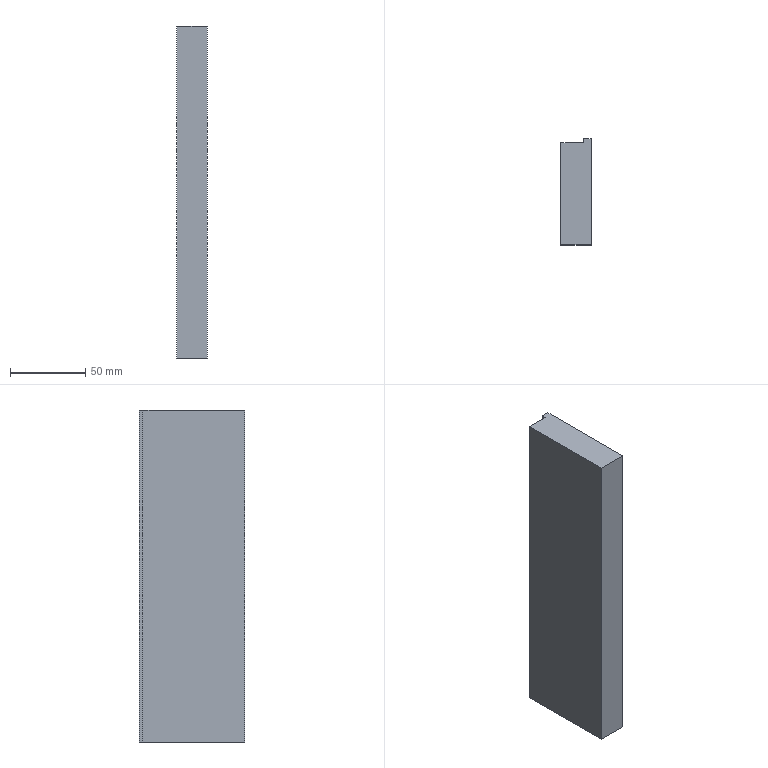Part | STEP file | Backup 2012-3-22-015 | 1 solid | 8 faces | box 20 x 70 x 220 mm | volume 299750 mm3 | plane 8
STEP:
#1=CARTESIAN_POINT('',(0.,0.,0.));
#2=DIRECTION('',(0.,0.,1.));
#3=DIRECTION('',(1.,0.,0.));
#4=AXIS2_PLACEMENT_3D('',#1,#2,#3);
#5=CARTESIAN_POINT('',(0.,67.5,0.));
#6=VERTEX_POINT('',#5);
#7=CARTESIAN_POINT('',(0.,0.,0.));
#8=VERTEX_POINT('',#7);
#9=CARTESIAN_POINT('',(0.,0.,0.));
#10=DIRECTION('',(0.,-1.,0.));
#11=VECTOR('',#10,1.);
#12=LINE('',#9,#11);
#13=CARTESIAN_POINT('',(0.,0.,220.));
#14=DIRECTION('',(1.,0.,0.));
#15=DIRECTION('',(0.,0.,-1.));
#16=AXIS2_PLACEMENT_3D('',#13,#14,#15);
#17=PLANE('',#16);
#18=CARTESIAN_POINT('',(220.,0.));
#19=DIRECTION('',(0.,-1.));
#20=VECTOR('',#19,1.);
#21=LINE('',#18,#20);
#22=(GEOMETRIC_REPRESENTATION_CONTEXT(2)PARAMETRIC_REPRESENTATION_CONTEXT()REPRESENTATION_CONTEXT('',''));
#23=DEFINITIONAL_REPRESENTATION('',(#21),#22);
#24=PCURVE('',#17,#23);
#25=CARTESIAN_POINT('',(0.,67.5,0.));
#26=DIRECTION('',(0.,0.,1.));
#27=DIRECTION('',(1.,0.,0.));
#28=AXIS2_PLACEMENT_3D('',#25,#26,#27);
#29=PLANE('',#28);
#30=CARTESIAN_POINT('',(0.,-67.5));
#31=DIRECTION('',(0.,-1.));
#32=VECTOR('',#31,1.);
#33=LINE('',#30,#32);
#34=(GEOMETRIC_REPRESENTATION_CONTEXT(2)PARAMETRIC_REPRESENTATION_CONTEXT()REPRESENTATION_CONTEXT('',''));
#35=DEFINITIONAL_REPRESENTATION('',(#33),#34);
#36=PCURVE('',#29,#35);
#37=SURFACE_CURVE('',#12,(#24,#36),.PCURVE_S1.);
#38=EDGE_CURVE('',#6,#8,#37,.T.);
#39=ORIENTED_EDGE('',*,*,#38,.T.);
#40=CARTESIAN_POINT('',(0.,0.,220.));
#41=VERTEX_POINT('',#40);
#42=CARTESIAN_POINT('',(0.,0.,220.));
#43=DIRECTION('',(0.,0.,-1.));
#44=VECTOR('',#43,1.);
#45=LINE('',#42,#44);
#46=CARTESIAN_POINT('',(0.,0.));
#47=DIRECTION('',(1.,0.));
#48=VECTOR('',#47,1.);
#49=LINE('',#46,#48);
#50=(GEOMETRIC_REPRESENTATION_CONTEXT(2)PARAMETRIC_REPRESENTATION_CONTEXT()REPRESENTATION_CONTEXT('',''));
#51=DEFINITIONAL_REPRESENTATION('',(#49),#50);
#52=PCURVE('',#17,#51);
#53=CARTESIAN_POINT('',(0.,0.,220.));
#54=DIRECTION('',(0.,1.,0.));
#55=DIRECTION('',(0.,0.,1.));
#56=AXIS2_PLACEMENT_3D('',#53,#54,#55);
#57=PLANE('',#56);
#58=CARTESIAN_POINT('',(0.,0.));
#59=DIRECTION('',(-1.,0.));
#60=VECTOR('',#59,1.);
#61=LINE('',#58,#60);
#62=(GEOMETRIC_REPRESENTATION_CONTEXT(2)PARAMETRIC_REPRESENTATION_CONTEXT()REPRESENTATION_CONTEXT('',''));
#63=DEFINITIONAL_REPRESENTATION('',(#61),#62);
#64=PCURVE('',#57,#63);
#65=SURFACE_CURVE('',#45,(#52,#64),.PCURVE_S1.);
#66=EDGE_CURVE('',#41,#8,#65,.T.);
#67=ORIENTED_EDGE('',*,*,#66,.F.);
#68=CARTESIAN_POINT('',(0.,67.5,220.));
#69=VERTEX_POINT('',#68);
#70=CARTESIAN_POINT('',(0.,0.,220.));
#71=DIRECTION('',(0.,-1.,0.));
#72=VECTOR('',#71,1.);
#73=LINE('',#70,#72);
#74=CARTESIAN_POINT('',(0.,0.));
#75=DIRECTION('',(0.,-1.));
#76=VECTOR('',#75,1.);
#77=LINE('',#74,#76);
#78=(GEOMETRIC_REPRESENTATION_CONTEXT(2)PARAMETRIC_REPRESENTATION_CONTEXT()REPRESENTATION_CONTEXT('',''));
#79=DEFINITIONAL_REPRESENTATION('',(#77),#78);
#80=PCURVE('',#17,#79);
#81=CARTESIAN_POINT('',(0.,67.5,220.));
#82=DIRECTION('',(0.,0.,1.));
#83=DIRECTION('',(1.,0.,0.));
#84=AXIS2_PLACEMENT_3D('',#81,#82,#83);
#85=PLANE('',#84);
#86=CARTESIAN_POINT('',(0.,-67.5));
#87=DIRECTION('',(0.,-1.));
#88=VECTOR('',#87,1.);
#89=LINE('',#86,#88);
#90=(GEOMETRIC_REPRESENTATION_CONTEXT(2)PARAMETRIC_REPRESENTATION_CONTEXT()REPRESENTATION_CONTEXT('',''));
#91=DEFINITIONAL_REPRESENTATION('',(#89),#90);
#92=PCURVE('',#85,#91);
#93=SURFACE_CURVE('',#73,(#80,#92),.PCURVE_S1.);
#94=EDGE_CURVE('',#69,#41,#93,.T.);
#95=ORIENTED_EDGE('',*,*,#94,.F.);
#96=CARTESIAN_POINT('',(0.,67.5,220.));
#97=DIRECTION('',(0.,0.,-1.));
#98=VECTOR('',#97,1.);
#99=LINE('',#96,#98);
#100=CARTESIAN_POINT('',(0.,67.5));
#101=DIRECTION('',(1.,0.));
#102=VECTOR('',#101,1.);
#103=LINE('',#100,#102);
#104=(GEOMETRIC_REPRESENTATION_CONTEXT(2)PARAMETRIC_REPRESENTATION_CONTEXT()REPRESENTATION_CONTEXT('',''));
#105=DEFINITIONAL_REPRESENTATION('',(#103),#104);
#106=PCURVE('',#17,#105);
#107=CARTESIAN_POINT('',(15.,67.5,220.));
#108=DIRECTION('',(0.,-1.,0.));
#109=DIRECTION('',(0.,0.,-1.));
#110=AXIS2_PLACEMENT_3D('',#107,#108,#109);
#111=PLANE('',#110);
#112=CARTESIAN_POINT('',(0.,-15.));
#113=DIRECTION('',(1.,0.));
#114=VECTOR('',#113,1.);
#115=LINE('',#112,#114);
#116=(GEOMETRIC_REPRESENTATION_CONTEXT(2)PARAMETRIC_REPRESENTATION_CONTEXT()REPRESENTATION_CONTEXT('',''));
#117=DEFINITIONAL_REPRESENTATION('',(#115),#116);
#118=PCURVE('',#111,#117);
#119=SURFACE_CURVE('',#99,(#106,#118),.PCURVE_S1.);
#120=EDGE_CURVE('',#69,#6,#119,.T.);
#121=ORIENTED_EDGE('',*,*,#120,.T.);
#122=EDGE_LOOP('',(#39,#67,#95,#121));
#123=FACE_BOUND('',#122,.T.);
#124=ADVANCED_FACE('',(#123),#17,.F.);
#125=CARTESIAN_POINT('',(20.,0.,0.));
#126=VERTEX_POINT('',#125);
#127=CARTESIAN_POINT('',(0.,0.,0.));
#128=DIRECTION('',(1.,0.,0.));
#129=VECTOR('',#128,1.);
#130=LINE('',#127,#129);
#131=CARTESIAN_POINT('',(-220.,0.));
#132=DIRECTION('',(0.,1.));
#133=VECTOR('',#132,1.);
#134=LINE('',#131,#133);
#135=(GEOMETRIC_REPRESENTATION_CONTEXT(2)PARAMETRIC_REPRESENTATION_CONTEXT()REPRESENTATION_CONTEXT('',''));
#136=DEFINITIONAL_REPRESENTATION('',(#134),#135);
#137=PCURVE('',#57,#136);
#138=CARTESIAN_POINT('',(0.,-67.5));
#139=DIRECTION('',(1.,0.));
#140=VECTOR('',#139,1.);
#141=LINE('',#138,#140);
#142=(GEOMETRIC_REPRESENTATION_CONTEXT(2)PARAMETRIC_REPRESENTATION_CONTEXT()REPRESENTATION_CONTEXT('',''));
#143=DEFINITIONAL_REPRESENTATION('',(#141),#142);
#144=PCURVE('',#29,#143);
#145=SURFACE_CURVE('',#130,(#137,#144),.PCURVE_S1.);
#146=EDGE_CURVE('',#8,#126,#145,.T.);
#147=ORIENTED_EDGE('',*,*,#146,.T.);
#148=CARTESIAN_POINT('',(20.,0.,220.));
#149=VERTEX_POINT('',#148);
#150=CARTESIAN_POINT('',(20.,0.,220.));
#151=DIRECTION('',(0.,0.,-1.));
#152=VECTOR('',#151,1.);
#153=LINE('',#150,#152);
#154=CARTESIAN_POINT('',(0.,20.));
#155=DIRECTION('',(-1.,0.));
#156=VECTOR('',#155,1.);
#157=LINE('',#154,#156);
#158=(GEOMETRIC_REPRESENTATION_CONTEXT(2)PARAMETRIC_REPRESENTATION_CONTEXT()REPRESENTATION_CONTEXT('',''));
#159=DEFINITIONAL_REPRESENTATION('',(#157),#158);
#160=PCURVE('',#57,#159);
#161=CARTESIAN_POINT('',(20.,0.,220.));
#162=DIRECTION('',(-1.,0.,0.));
#163=DIRECTION('',(0.,-1.,0.));
#164=AXIS2_PLACEMENT_3D('',#161,#162,#163);
#165=PLANE('',#164);
#166=CARTESIAN_POINT('',(0.,0.));
#167=DIRECTION('',(0.,-1.));
#168=VECTOR('',#167,1.);
#169=LINE('',#166,#168);
#170=(GEOMETRIC_REPRESENTATION_CONTEXT(2)PARAMETRIC_REPRESENTATION_CONTEXT()REPRESENTATION_CONTEXT('',''));
#171=DEFINITIONAL_REPRESENTATION('',(#169),#170);
#172=PCURVE('',#165,#171);
#173=SURFACE_CURVE('',#153,(#160,#172),.PCURVE_S1.);
#174=EDGE_CURVE('',#149,#126,#173,.T.);
#175=ORIENTED_EDGE('',*,*,#174,.F.);
#176=CARTESIAN_POINT('',(0.,0.,220.));
#177=DIRECTION('',(1.,0.,0.));
#178=VECTOR('',#177,1.);
#179=LINE('',#176,#178);
#180=CARTESIAN_POINT('',(0.,0.));
#181=DIRECTION('',(0.,1.));
#182=VECTOR('',#181,1.);
#183=LINE('',#180,#182);
#184=(GEOMETRIC_REPRESENTATION_CONTEXT(2)PARAMETRIC_REPRESENTATION_CONTEXT()REPRESENTATION_CONTEXT('',''));
#185=DEFINITIONAL_REPRESENTATION('',(#183),#184);
#186=PCURVE('',#57,#185);
#187=CARTESIAN_POINT('',(0.,-67.5));
#188=DIRECTION('',(1.,0.));
#189=VECTOR('',#188,1.);
#190=LINE('',#187,#189);
#191=(GEOMETRIC_REPRESENTATION_CONTEXT(2)PARAMETRIC_REPRESENTATION_CONTEXT()REPRESENTATION_CONTEXT('',''));
#192=DEFINITIONAL_REPRESENTATION('',(#190),#191);
#193=PCURVE('',#85,#192);
#194=SURFACE_CURVE('',#179,(#186,#193),.PCURVE_S1.);
#195=EDGE_CURVE('',#41,#149,#194,.T.);
#196=ORIENTED_EDGE('',*,*,#195,.F.);
#197=ORIENTED_EDGE('',*,*,#66,.T.);
#198=EDGE_LOOP('',(#147,#175,#196,#197));
#199=FACE_BOUND('',#198,.T.);
#200=ADVANCED_FACE('',(#199),#57,.F.);
#201=CARTESIAN_POINT('',(20.,70.,0.));
#202=VERTEX_POINT('',#201);
#203=CARTESIAN_POINT('',(20.,0.,0.));
#204=DIRECTION('',(0.,1.,0.));
#205=VECTOR('',#204,1.);
#206=LINE('',#203,#205);
#207=CARTESIAN_POINT('',(0.,-220.));
#208=DIRECTION('',(-1.,0.));
#209=VECTOR('',#208,1.);
#210=LINE('',#207,#209);
#211=(GEOMETRIC_REPRESENTATION_CONTEXT(2)PARAMETRIC_REPRESENTATION_CONTEXT()REPRESENTATION_CONTEXT('',''));
#212=DEFINITIONAL_REPRESENTATION('',(#210),#211);
#213=PCURVE('',#165,#212);
#214=CARTESIAN_POINT('',(20.,-67.5));
#215=DIRECTION('',(0.,1.));
#216=VECTOR('',#215,1.);
#217=LINE('',#214,#216);
#218=(GEOMETRIC_REPRESENTATION_CONTEXT(2)PARAMETRIC_REPRESENTATION_CONTEXT()REPRESENTATION_CONTEXT('',''));
#219=DEFINITIONAL_REPRESENTATION('',(#217),#218);
#220=PCURVE('',#29,#219);
#221=SURFACE_CURVE('',#206,(#213,#220),.PCURVE_S1.);
#222=EDGE_CURVE('',#126,#202,#221,.T.);
#223=ORIENTED_EDGE('',*,*,#222,.T.);
#224=CARTESIAN_POINT('',(20.,70.,220.));
#225=VERTEX_POINT('',#224);
#226=CARTESIAN_POINT('',(20.,70.,220.));
#227=DIRECTION('',(0.,0.,-1.));
#228=VECTOR('',#227,1.);
#229=LINE('',#226,#228);
#230=CARTESIAN_POINT('',(-70.,0.));
#231=DIRECTION('',(0.,-1.));
#232=VECTOR('',#231,1.);
#233=LINE('',#230,#232);
#234=(GEOMETRIC_REPRESENTATION_CONTEXT(2)PARAMETRIC_REPRESENTATION_CONTEXT()REPRESENTATION_CONTEXT('',''));
#235=DEFINITIONAL_REPRESENTATION('',(#233),#234);
#236=PCURVE('',#165,#235);
#237=CARTESIAN_POINT('',(15.,70.,220.));
#238=DIRECTION('',(0.,-1.,0.));
#239=DIRECTION('',(0.,0.,-1.));
#240=AXIS2_PLACEMENT_3D('',#237,#238,#239);
#241=PLANE('',#240);
#242=CARTESIAN_POINT('',(0.,5.));
#243=DIRECTION('',(1.,0.));
#244=VECTOR('',#243,1.);
#245=LINE('',#242,#244);
#246=(GEOMETRIC_REPRESENTATION_CONTEXT(2)PARAMETRIC_REPRESENTATION_CONTEXT()REPRESENTATION_CONTEXT('',''));
#247=DEFINITIONAL_REPRESENTATION('',(#245),#246);
#248=PCURVE('',#241,#247);
#249=SURFACE_CURVE('',#229,(#236,#248),.PCURVE_S1.);
#250=EDGE_CURVE('',#225,#202,#249,.T.);
#251=ORIENTED_EDGE('',*,*,#250,.F.);
#252=CARTESIAN_POINT('',(20.,0.,220.));
#253=DIRECTION('',(0.,1.,0.));
#254=VECTOR('',#253,1.);
#255=LINE('',#252,#254);
#256=CARTESIAN_POINT('',(0.,0.));
#257=DIRECTION('',(-1.,0.));
#258=VECTOR('',#257,1.);
#259=LINE('',#256,#258);
#260=(GEOMETRIC_REPRESENTATION_CONTEXT(2)PARAMETRIC_REPRESENTATION_CONTEXT()REPRESENTATION_CONTEXT('',''));
#261=DEFINITIONAL_REPRESENTATION('',(#259),#260);
#262=PCURVE('',#165,#261);
#263=CARTESIAN_POINT('',(20.,-67.5));
#264=DIRECTION('',(0.,1.));
#265=VECTOR('',#264,1.);
#266=LINE('',#263,#265);
#267=(GEOMETRIC_REPRESENTATION_CONTEXT(2)PARAMETRIC_REPRESENTATION_CONTEXT()REPRESENTATION_CONTEXT('',''));
#268=DEFINITIONAL_REPRESENTATION('',(#266),#267);
#269=PCURVE('',#85,#268);
#270=SURFACE_CURVE('',#255,(#262,#269),.PCURVE_S1.);
#271=EDGE_CURVE('',#149,#225,#270,.T.);
#272=ORIENTED_EDGE('',*,*,#271,.F.);
#273=ORIENTED_EDGE('',*,*,#174,.T.);
#274=EDGE_LOOP('',(#223,#251,#272,#273));
#275=FACE_BOUND('',#274,.T.);
#276=ADVANCED_FACE('',(#275),#165,.F.);
#277=CARTESIAN_POINT('',(15.,70.,0.));
#278=VERTEX_POINT('',#277);
#279=CARTESIAN_POINT('',(15.,70.,0.));
#280=DIRECTION('',(-1.,0.,0.));
#281=VECTOR('',#280,1.);
#282=LINE('',#279,#281);
#283=CARTESIAN_POINT('',(220.,0.));
#284=DIRECTION('',(0.,-1.));
#285=VECTOR('',#284,1.);
#286=LINE('',#283,#285);
#287=(GEOMETRIC_REPRESENTATION_CONTEXT(2)PARAMETRIC_REPRESENTATION_CONTEXT()REPRESENTATION_CONTEXT('',''));
#288=DEFINITIONAL_REPRESENTATION('',(#286),#287);
#289=PCURVE('',#241,#288);
#290=CARTESIAN_POINT('',(15.,2.5));
#291=DIRECTION('',(-1.,0.));
#292=VECTOR('',#291,1.);
#293=LINE('',#290,#292);
#294=(GEOMETRIC_REPRESENTATION_CONTEXT(2)PARAMETRIC_REPRESENTATION_CONTEXT()REPRESENTATION_CONTEXT('',''));
#295=DEFINITIONAL_REPRESENTATION('',(#293),#294);
#296=PCURVE('',#29,#295);
#297=SURFACE_CURVE('',#282,(#289,#296),.PCURVE_S1.);
#298=EDGE_CURVE('',#202,#278,#297,.T.);
#299=ORIENTED_EDGE('',*,*,#298,.T.);
#300=CARTESIAN_POINT('',(15.,70.,220.));
#301=VERTEX_POINT('',#300);
#302=CARTESIAN_POINT('',(15.,70.,220.));
#303=DIRECTION('',(0.,0.,-1.));
#304=VECTOR('',#303,1.);
#305=LINE('',#302,#304);
#306=CARTESIAN_POINT('',(0.,0.));
#307=DIRECTION('',(1.,0.));
#308=VECTOR('',#307,1.);
#309=LINE('',#306,#308);
#310=(GEOMETRIC_REPRESENTATION_CONTEXT(2)PARAMETRIC_REPRESENTATION_CONTEXT()REPRESENTATION_CONTEXT('',''));
#311=DEFINITIONAL_REPRESENTATION('',(#309),#310);
#312=PCURVE('',#241,#311);
#313=CARTESIAN_POINT('',(15.,70.,220.));
#314=DIRECTION('',(1.,0.,0.));
#315=DIRECTION('',(0.,0.,-1.));
#316=AXIS2_PLACEMENT_3D('',#313,#314,#315);
#317=PLANE('',#316);
#318=CARTESIAN_POINT('',(0.,0.));
#319=DIRECTION('',(1.,0.));
#320=VECTOR('',#319,1.);
#321=LINE('',#318,#320);
#322=(GEOMETRIC_REPRESENTATION_CONTEXT(2)PARAMETRIC_REPRESENTATION_CONTEXT()REPRESENTATION_CONTEXT('',''));
#323=DEFINITIONAL_REPRESENTATION('',(#321),#322);
#324=PCURVE('',#317,#323);
#325=SURFACE_CURVE('',#305,(#312,#324),.PCURVE_S1.);
#326=EDGE_CURVE('',#301,#278,#325,.T.);
#327=ORIENTED_EDGE('',*,*,#326,.F.);
#328=CARTESIAN_POINT('',(15.,70.,220.));
#329=DIRECTION('',(-1.,0.,0.));
#330=VECTOR('',#329,1.);
#331=LINE('',#328,#330);
#332=CARTESIAN_POINT('',(0.,0.));
#333=DIRECTION('',(0.,-1.));
#334=VECTOR('',#333,1.);
#335=LINE('',#332,#334);
#336=(GEOMETRIC_REPRESENTATION_CONTEXT(2)PARAMETRIC_REPRESENTATION_CONTEXT()REPRESENTATION_CONTEXT('',''));
#337=DEFINITIONAL_REPRESENTATION('',(#335),#336);
#338=PCURVE('',#241,#337);
#339=CARTESIAN_POINT('',(15.,2.5));
#340=DIRECTION('',(-1.,0.));
#341=VECTOR('',#340,1.);
#342=LINE('',#339,#341);
#343=(GEOMETRIC_REPRESENTATION_CONTEXT(2)PARAMETRIC_REPRESENTATION_CONTEXT()REPRESENTATION_CONTEXT('',''));
#344=DEFINITIONAL_REPRESENTATION('',(#342),#343);
#345=PCURVE('',#85,#344);
#346=SURFACE_CURVE('',#331,(#338,#345),.PCURVE_S1.);
#347=EDGE_CURVE('',#225,#301,#346,.T.);
#348=ORIENTED_EDGE('',*,*,#347,.F.);
#349=ORIENTED_EDGE('',*,*,#250,.T.);
#350=EDGE_LOOP('',(#299,#327,#348,#349));
#351=FACE_BOUND('',#350,.T.);
#352=ADVANCED_FACE('',(#351),#241,.F.);
#353=CARTESIAN_POINT('',(15.,67.5,0.));
#354=VERTEX_POINT('',#353);
#355=CARTESIAN_POINT('',(15.,70.,0.));
#356=DIRECTION('',(0.,-1.,0.));
#357=VECTOR('',#356,1.);
#358=LINE('',#355,#357);
#359=CARTESIAN_POINT('',(220.,0.));
#360=DIRECTION('',(0.,-1.));
#361=VECTOR('',#360,1.);
#362=LINE('',#359,#361);
#363=(GEOMETRIC_REPRESENTATION_CONTEXT(2)PARAMETRIC_REPRESENTATION_CONTEXT()REPRESENTATION_CONTEXT('',''));
#364=DEFINITIONAL_REPRESENTATION('',(#362),#363);
#365=PCURVE('',#317,#364);
#366=CARTESIAN_POINT('',(15.,2.5));
#367=DIRECTION('',(0.,-1.));
#368=VECTOR('',#367,1.);
#369=LINE('',#366,#368);
#370=(GEOMETRIC_REPRESENTATION_CONTEXT(2)PARAMETRIC_REPRESENTATION_CONTEXT()REPRESENTATION_CONTEXT('',''));
#371=DEFINITIONAL_REPRESENTATION('',(#369),#370);
#372=PCURVE('',#29,#371);
#373=SURFACE_CURVE('',#358,(#365,#372),.PCURVE_S1.);
#374=EDGE_CURVE('',#278,#354,#373,.T.);
#375=ORIENTED_EDGE('',*,*,#374,.T.);
#376=CARTESIAN_POINT('',(15.,67.5,220.));
#377=VERTEX_POINT('',#376);
#378=CARTESIAN_POINT('',(15.,67.5,220.));
#379=DIRECTION('',(0.,0.,-1.));
#380=VECTOR('',#379,1.);
#381=LINE('',#378,#380);
#382=CARTESIAN_POINT('',(0.,-2.5));
#383=DIRECTION('',(1.,0.));
#384=VECTOR('',#383,1.);
#385=LINE('',#382,#384);
#386=(GEOMETRIC_REPRESENTATION_CONTEXT(2)PARAMETRIC_REPRESENTATION_CONTEXT()REPRESENTATION_CONTEXT('',''));
#387=DEFINITIONAL_REPRESENTATION('',(#385),#386);
#388=PCURVE('',#317,#387);
#389=CARTESIAN_POINT('',(0.,0.));
#390=DIRECTION('',(1.,0.));
#391=VECTOR('',#390,1.);
#392=LINE('',#389,#391);
#393=(GEOMETRIC_REPRESENTATION_CONTEXT(2)PARAMETRIC_REPRESENTATION_CONTEXT()REPRESENTATION_CONTEXT('',''));
#394=DEFINITIONAL_REPRESENTATION('',(#392),#393);
#395=PCURVE('',#111,#394);
#396=SURFACE_CURVE('',#381,(#388,#395),.PCURVE_S1.);
#397=EDGE_CURVE('',#377,#354,#396,.T.);
#398=ORIENTED_EDGE('',*,*,#397,.F.);
#399=CARTESIAN_POINT('',(15.,70.,220.));
#400=DIRECTION('',(0.,-1.,0.));
#401=VECTOR('',#400,1.);
#402=LINE('',#399,#401);
#403=CARTESIAN_POINT('',(0.,0.));
#404=DIRECTION('',(0.,-1.));
#405=VECTOR('',#404,1.);
#406=LINE('',#403,#405);
#407=(GEOMETRIC_REPRESENTATION_CONTEXT(2)PARAMETRIC_REPRESENTATION_CONTEXT()REPRESENTATION_CONTEXT('',''));
#408=DEFINITIONAL_REPRESENTATION('',(#406),#407);
#409=PCURVE('',#317,#408);
#410=CARTESIAN_POINT('',(15.,2.5));
#411=DIRECTION('',(0.,-1.));
#412=VECTOR('',#411,1.);
#413=LINE('',#410,#412);
#414=(GEOMETRIC_REPRESENTATION_CONTEXT(2)PARAMETRIC_REPRESENTATION_CONTEXT()REPRESENTATION_CONTEXT('',''));
#415=DEFINITIONAL_REPRESENTATION('',(#413),#414);
#416=PCURVE('',#85,#415);
#417=SURFACE_CURVE('',#402,(#409,#416),.PCURVE_S1.);
#418=EDGE_CURVE('',#301,#377,#417,.T.);
#419=ORIENTED_EDGE('',*,*,#418,.F.);
#420=ORIENTED_EDGE('',*,*,#326,.T.);
#421=EDGE_LOOP('',(#375,#398,#419,#420));
#422=FACE_BOUND('',#421,.T.);
#423=ADVANCED_FACE('',(#422),#317,.F.);
#424=CARTESIAN_POINT('',(15.,67.5,0.));
#425=DIRECTION('',(-1.,0.,0.));
#426=VECTOR('',#425,1.);
#427=LINE('',#424,#426);
#428=CARTESIAN_POINT('',(220.,0.));
#429=DIRECTION('',(0.,-1.));
#430=VECTOR('',#429,1.);
#431=LINE('',#428,#430);
#432=(GEOMETRIC_REPRESENTATION_CONTEXT(2)PARAMETRIC_REPRESENTATION_CONTEXT()REPRESENTATION_CONTEXT('',''));
#433=DEFINITIONAL_REPRESENTATION('',(#431),#432);
#434=PCURVE('',#111,#433);
#435=CARTESIAN_POINT('',(15.,0.));
#436=DIRECTION('',(-1.,0.));
#437=VECTOR('',#436,1.);
#438=LINE('',#435,#437);
#439=(GEOMETRIC_REPRESENTATION_CONTEXT(2)PARAMETRIC_REPRESENTATION_CONTEXT()REPRESENTATION_CONTEXT('',''));
#440=DEFINITIONAL_REPRESENTATION('',(#438),#439);
#441=PCURVE('',#29,#440);
#442=SURFACE_CURVE('',#427,(#434,#441),.PCURVE_S1.);
#443=EDGE_CURVE('',#354,#6,#442,.T.);
#444=ORIENTED_EDGE('',*,*,#443,.T.);
#445=ORIENTED_EDGE('',*,*,#120,.F.);
#446=CARTESIAN_POINT('',(15.,67.5,220.));
#447=DIRECTION('',(-1.,0.,0.));
#448=VECTOR('',#447,1.);
#449=LINE('',#446,#448);
#450=CARTESIAN_POINT('',(0.,0.));
#451=DIRECTION('',(0.,-1.));
#452=VECTOR('',#451,1.);
#453=LINE('',#450,#452);
#454=(GEOMETRIC_REPRESENTATION_CONTEXT(2)PARAMETRIC_REPRESENTATION_CONTEXT()REPRESENTATION_CONTEXT('',''));
#455=DEFINITIONAL_REPRESENTATION('',(#453),#454);
#456=PCURVE('',#111,#455);
#457=CARTESIAN_POINT('',(15.,0.));
#458=DIRECTION('',(-1.,0.));
#459=VECTOR('',#458,1.);
#460=LINE('',#457,#459);
#461=(GEOMETRIC_REPRESENTATION_CONTEXT(2)PARAMETRIC_REPRESENTATION_CONTEXT()REPRESENTATION_CONTEXT('',''));
#462=DEFINITIONAL_REPRESENTATION('',(#460),#461);
#463=PCURVE('',#85,#462);
#464=SURFACE_CURVE('',#449,(#456,#463),.PCURVE_S1.);
#465=EDGE_CURVE('',#377,#69,#464,.T.);
#466=ORIENTED_EDGE('',*,*,#465,.F.);
#467=ORIENTED_EDGE('',*,*,#397,.T.);
#468=EDGE_LOOP('',(#444,#445,#466,#467));
#469=FACE_BOUND('',#468,.T.);
#470=ADVANCED_FACE('',(#469),#111,.F.);
#471=ORIENTED_EDGE('',*,*,#94,.T.);
#472=ORIENTED_EDGE('',*,*,#195,.T.);
#473=ORIENTED_EDGE('',*,*,#271,.T.);
#474=ORIENTED_EDGE('',*,*,#347,.T.);
#475=ORIENTED_EDGE('',*,*,#418,.T.);
#476=ORIENTED_EDGE('',*,*,#465,.T.);
#477=EDGE_LOOP('',(#471,#472,#473,#474,#475,#476));
#478=FACE_BOUND('',#477,.T.);
#479=ADVANCED_FACE('',(#478),#85,.T.);
#480=ORIENTED_EDGE('',*,*,#38,.F.);
#481=ORIENTED_EDGE('',*,*,#443,.F.);
#482=ORIENTED_EDGE('',*,*,#374,.F.);
#483=ORIENTED_EDGE('',*,*,#298,.F.);
#484=ORIENTED_EDGE('',*,*,#222,.F.);
#485=ORIENTED_EDGE('',*,*,#146,.F.);
#486=EDGE_LOOP('',(#480,#481,#482,#483,#484,#485));
#487=FACE_BOUND('',#486,.T.);
#488=ADVANCED_FACE('',(#487),#29,.F.);
#489=CLOSED_SHELL('',(#124,#200,#276,#352,#423,#470,#479,#488));
#490=MANIFOLD_SOLID_BREP('',#489);
#491=(LENGTH_UNIT()NAMED_UNIT(*)SI_UNIT(.MILLI.,.METRE.));
#492=UNCERTAINTY_MEASURE_WITH_UNIT(LENGTH_MEASURE(0.0000001),#491,'','');
#493=(NAMED_UNIT(*)PLANE_ANGLE_UNIT()SI_UNIT($,.RADIAN.));
#494=(NAMED_UNIT(*)SI_UNIT($,.STERADIAN.)SOLID_ANGLE_UNIT());
#495=(GEOMETRIC_REPRESENTATION_CONTEXT(3)GLOBAL_UNCERTAINTY_ASSIGNED_CONTEXT((#492))GLOBAL_UNIT_ASSIGNED_CONTEXT((#491,#493,#494))REPRESENTATION_CONTEXT('',''));
#496=ADVANCED_BREP_SHAPE_REPRESENTATION('',(#4,#490),#495);